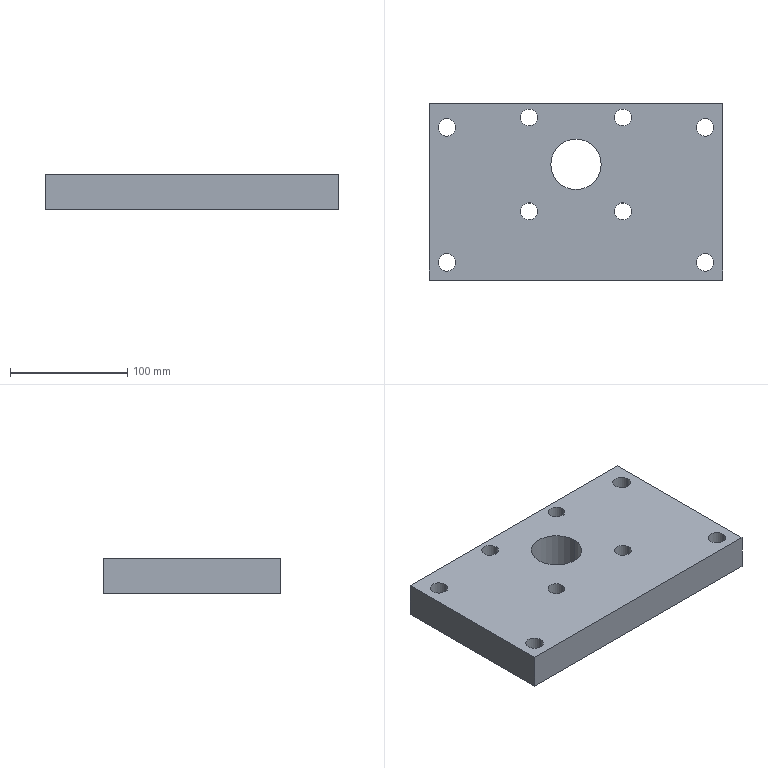Part | STEP file | TAM GA XYLANH GIUA_3 | 1 solid | 24 faces | box 250 x 150 x 30 mm | volume 1040750 mm3 | cylinder 18 | plane 6 | commonest cylinder face diameters 14.376 x8 15 x8 43 x2